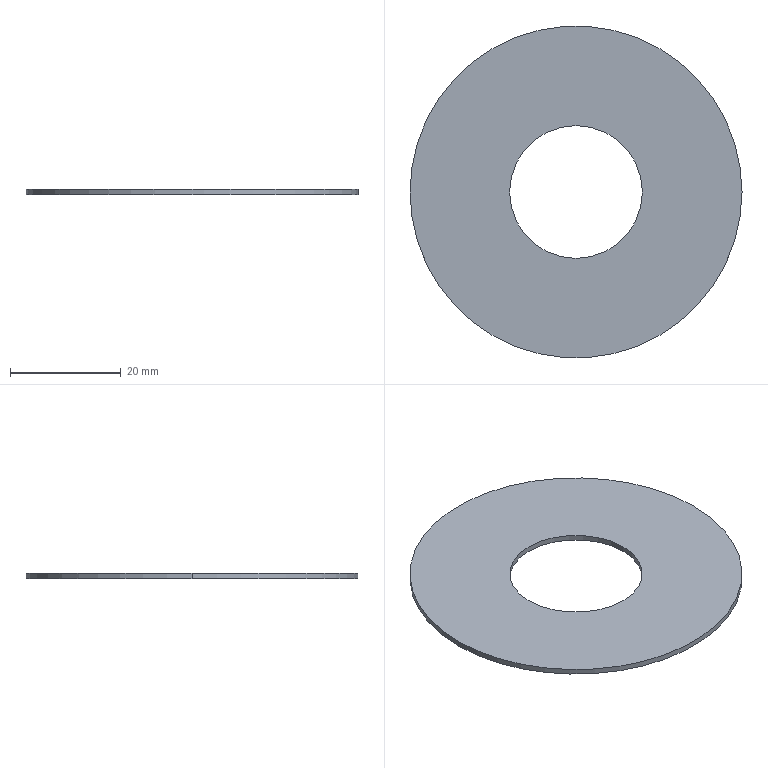Part | SolidWorks | features ImportedCurve 16, BaseBody 1 | 1 solid | 6 faces | box 60 x 60 x 1 mm | volume 2375 mm3 | cylinder 4 | plane 2 | commonest cylinder face diameters 24 x2 60 x2
STEP:
#1=CARTESIAN_POINT('',(12.,0.,0.));
#2=VERTEX_POINT('',#1);
#3=CARTESIAN_POINT('',(12.,0.,1.));
#4=VERTEX_POINT('',#3);
#5=CARTESIAN_POINT('',(12.,0.,0.));
#6=DIRECTION('',(0.,0.,1.));
#7=VECTOR('',#6,1000.);
#8=LINE('',#5,#7);
#9=EDGE_CURVE('',#2,#4,#8,.T.);
#10=ORIENTED_EDGE('',*,*,#9,.T.);
#11=CARTESIAN_POINT('',(-12.,0.,1.));
#12=VERTEX_POINT('',#11);
#13=CARTESIAN_POINT('',(0.,0.,1.));
#14=DIRECTION('',(0.,0.,-1.));
#15=DIRECTION('',(-1.,0.,0.));
#16=AXIS2_PLACEMENT_3D('',#13,#14,#15);
#17=CIRCLE('',#16,12.);
#18=EDGE_CURVE('',#12,#4,#17,.T.);
#19=ORIENTED_EDGE('',*,*,#18,.F.);
#20=CARTESIAN_POINT('',(-12.,0.,0.));
#21=VERTEX_POINT('',#20);
#22=CARTESIAN_POINT('',(-12.,0.,0.));
#23=DIRECTION('',(0.,0.,1.));
#24=VECTOR('',#23,1000.);
#25=LINE('',#22,#24);
#26=EDGE_CURVE('',#21,#12,#25,.T.);
#27=ORIENTED_EDGE('',*,*,#26,.F.);
#28=CARTESIAN_POINT('',(0.,0.,0.));
#29=DIRECTION('',(0.,0.,-1.));
#30=DIRECTION('',(-1.,0.,0.));
#31=AXIS2_PLACEMENT_3D('',#28,#29,#30);
#32=CIRCLE('',#31,12.);
#33=EDGE_CURVE('',#21,#2,#32,.T.);
#34=ORIENTED_EDGE('',*,*,#33,.T.);
#35=EDGE_LOOP('',(#10,#19,#27,#34));
#36=FACE_OUTER_BOUND('',#35,.T.);
#37=CARTESIAN_POINT('',(0.,0.,0.));
#38=DIRECTION('',(0.,0.,1.));
#39=DIRECTION('',(1.,0.,0.));
#40=AXIS2_PLACEMENT_3D('',#37,#38,#39);
#41=CYLINDRICAL_SURFACE('',#40,12.);
#42=ADVANCED_FACE('',(#36),#41,.F.);
#43=ORIENTED_EDGE('',*,*,#26,.T.);
#44=CARTESIAN_POINT('',(0.,0.,1.));
#45=DIRECTION('',(0.,0.,-1.));
#46=DIRECTION('',(1.,0.,0.));
#47=AXIS2_PLACEMENT_3D('',#44,#45,#46);
#48=CIRCLE('',#47,12.);
#49=EDGE_CURVE('',#4,#12,#48,.T.);
#50=ORIENTED_EDGE('',*,*,#49,.F.);
#51=ORIENTED_EDGE('',*,*,#9,.F.);
#52=CARTESIAN_POINT('',(0.,0.,0.));
#53=DIRECTION('',(0.,0.,-1.));
#54=DIRECTION('',(1.,0.,0.));
#55=AXIS2_PLACEMENT_3D('',#52,#53,#54);
#56=CIRCLE('',#55,12.);
#57=EDGE_CURVE('',#2,#21,#56,.T.);
#58=ORIENTED_EDGE('',*,*,#57,.T.);
#59=EDGE_LOOP('',(#43,#50,#51,#58));
#60=FACE_OUTER_BOUND('',#59,.T.);
#61=CARTESIAN_POINT('',(0.,0.,0.));
#62=DIRECTION('',(0.,0.,1.));
#63=DIRECTION('',(1.,0.,0.));
#64=AXIS2_PLACEMENT_3D('',#61,#62,#63);
#65=CYLINDRICAL_SURFACE('',#64,12.);
#66=ADVANCED_FACE('',(#60),#65,.F.);
#67=ORIENTED_EDGE('',*,*,#18,.T.);
#68=ORIENTED_EDGE('',*,*,#49,.T.);
#69=EDGE_LOOP('',(#67,#68));
#70=FACE_BOUND('',#69,.T.);
#71=CARTESIAN_POINT('',(-30.,0.,1.));
#72=VERTEX_POINT('',#71);
#73=CARTESIAN_POINT('',(30.,0.,1.));
#74=VERTEX_POINT('',#73);
#75=CARTESIAN_POINT('',(0.,0.,1.));
#76=DIRECTION('',(0.,0.,1.));
#77=DIRECTION('',(-1.,0.,0.));
#78=AXIS2_PLACEMENT_3D('',#75,#76,#77);
#79=CIRCLE('',#78,30.);
#80=EDGE_CURVE('',#72,#74,#79,.T.);
#81=ORIENTED_EDGE('',*,*,#80,.T.);
#82=CARTESIAN_POINT('',(0.,0.,1.));
#83=DIRECTION('',(0.,0.,1.));
#84=DIRECTION('',(1.,0.,0.));
#85=AXIS2_PLACEMENT_3D('',#82,#83,#84);
#86=CIRCLE('',#85,30.);
#87=EDGE_CURVE('',#74,#72,#86,.T.);
#88=ORIENTED_EDGE('',*,*,#87,.T.);
#89=EDGE_LOOP('',(#81,#88));
#90=FACE_OUTER_BOUND('',#89,.T.);
#91=CARTESIAN_POINT('',(0.,0.,1.));
#92=DIRECTION('',(0.,0.,1.));
#93=DIRECTION('',(1.,0.,0.));
#94=AXIS2_PLACEMENT_3D('',#91,#92,#93);
#95=PLANE('',#94);
#96=ADVANCED_FACE('',(#70,#90),#95,.T.);
#97=CARTESIAN_POINT('',(30.,0.,0.));
#98=VERTEX_POINT('',#97);
#99=CARTESIAN_POINT('',(30.,0.,0.));
#100=DIRECTION('',(0.,0.,1.));
#101=VECTOR('',#100,1000.);
#102=LINE('',#99,#101);
#103=EDGE_CURVE('',#98,#74,#102,.T.);
#104=ORIENTED_EDGE('',*,*,#103,.T.);
#105=ORIENTED_EDGE('',*,*,#80,.F.);
#106=CARTESIAN_POINT('',(-30.,0.,0.));
#107=VERTEX_POINT('',#106);
#108=CARTESIAN_POINT('',(-30.,0.,0.));
#109=DIRECTION('',(0.,0.,1.));
#110=VECTOR('',#109,1000.);
#111=LINE('',#108,#110);
#112=EDGE_CURVE('',#107,#72,#111,.T.);
#113=ORIENTED_EDGE('',*,*,#112,.F.);
#114=CARTESIAN_POINT('',(0.,0.,0.));
#115=DIRECTION('',(0.,0.,1.));
#116=DIRECTION('',(-1.,0.,0.));
#117=AXIS2_PLACEMENT_3D('',#114,#115,#116);
#118=CIRCLE('',#117,30.);
#119=EDGE_CURVE('',#107,#98,#118,.T.);
#120=ORIENTED_EDGE('',*,*,#119,.T.);
#121=EDGE_LOOP('',(#104,#105,#113,#120));
#122=FACE_OUTER_BOUND('',#121,.T.);
#123=CARTESIAN_POINT('',(0.,0.,0.));
#124=DIRECTION('',(0.,0.,1.));
#125=DIRECTION('',(1.,0.,0.));
#126=AXIS2_PLACEMENT_3D('',#123,#124,#125);
#127=CYLINDRICAL_SURFACE('',#126,30.);
#128=ADVANCED_FACE('',(#122),#127,.T.);
#129=ORIENTED_EDGE('',*,*,#112,.T.);
#130=ORIENTED_EDGE('',*,*,#87,.F.);
#131=ORIENTED_EDGE('',*,*,#103,.F.);
#132=CARTESIAN_POINT('',(0.,0.,0.));
#133=DIRECTION('',(0.,0.,1.));
#134=DIRECTION('',(1.,0.,0.));
#135=AXIS2_PLACEMENT_3D('',#132,#133,#134);
#136=CIRCLE('',#135,30.);
#137=EDGE_CURVE('',#98,#107,#136,.T.);
#138=ORIENTED_EDGE('',*,*,#137,.T.);
#139=EDGE_LOOP('',(#129,#130,#131,#138));
#140=FACE_OUTER_BOUND('',#139,.T.);
#141=CARTESIAN_POINT('',(0.,0.,0.));
#142=DIRECTION('',(0.,0.,1.));
#143=DIRECTION('',(1.,0.,0.));
#144=AXIS2_PLACEMENT_3D('',#141,#142,#143);
#145=CYLINDRICAL_SURFACE('',#144,30.);
#146=ADVANCED_FACE('',(#140),#145,.T.);
#147=ORIENTED_EDGE('',*,*,#33,.F.);
#148=ORIENTED_EDGE('',*,*,#57,.F.);
#149=EDGE_LOOP('',(#147,#148));
#150=FACE_BOUND('',#149,.T.);
#151=ORIENTED_EDGE('',*,*,#119,.F.);
#152=ORIENTED_EDGE('',*,*,#137,.F.);
#153=EDGE_LOOP('',(#151,#152));
#154=FACE_OUTER_BOUND('',#153,.T.);
#155=CARTESIAN_POINT('',(0.,0.,0.));
#156=DIRECTION('',(0.,0.,1.));
#157=DIRECTION('',(1.,0.,0.));
#158=AXIS2_PLACEMENT_3D('',#155,#156,#157);
#159=PLANE('',#158);
#160=ADVANCED_FACE('',(#150,#154),#159,.F.);
#161=CLOSED_SHELL('',(#42,#66,#96,#128,#146,#160));
#162=MANIFOLD_SOLID_BREP('',#161);
#163=CARTESIAN_POINT('',(0.,0.,0.));
#164=DIRECTION('',(0.,0.,1.));
#165=DIRECTION('',(1.,0.,0.));
#166=AXIS2_PLACEMENT_3D('',#163,#164,#165);
#167=(LENGTH_UNIT()NAMED_UNIT(*)SI_UNIT(.MILLI.,.METRE.));
#168=UNCERTAINTY_MEASURE_WITH_UNIT(LENGTH_MEASURE(0.00001),#167,'','');
#169=(NAMED_UNIT(*)PLANE_ANGLE_UNIT()SI_UNIT($,.RADIAN.));
#170=(NAMED_UNIT(*)SI_UNIT($,.STERADIAN.)SOLID_ANGLE_UNIT());
#171=(GEOMETRIC_REPRESENTATION_CONTEXT(3)GLOBAL_UNCERTAINTY_ASSIGNED_CONTEXT((#168))GLOBAL_UNIT_ASSIGNED_CONTEXT((#167,#169,#170))REPRESENTATION_CONTEXT('',''));
#172=ADVANCED_BREP_SHAPE_REPRESENTATION('',(#162,#166),#171);